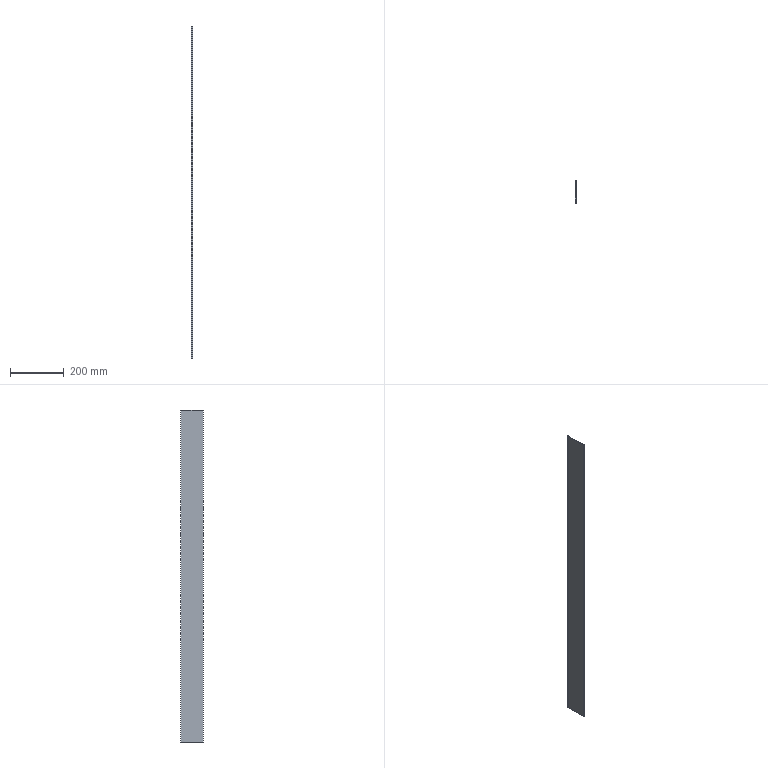Part | SolidWorks | features BaseBody 1 | 1 solid | 26 faces | box 4 x 85 x 1230 mm | volume 218982 mm3 | plane 18 | cylinder 8 | commonest cylinder face diameters 0.4 x4 1 x4
STEP:
#1=CARTESIAN_POINT('',(0.,0.,1230.));
#2=VERTEX_POINT('',#1);
#3=CARTESIAN_POINT('',(0.,0.,0.));
#4=VERTEX_POINT('',#3);
#5=CARTESIAN_POINT('',(0.,0.,1230.));
#6=DIRECTION('',(0.,0.,-1.));
#7=VECTOR('',#6,1000.);
#8=LINE('',#5,#7);
#9=EDGE_CURVE('',#2,#4,#8,.T.);
#10=ORIENTED_EDGE('',*,*,#9,.F.);
#11=CARTESIAN_POINT('',(0.,85.,1230.));
#12=VERTEX_POINT('',#11);
#13=CARTESIAN_POINT('',(0.,0.,1230.));
#14=DIRECTION('',(0.,-1.,0.));
#15=VECTOR('',#14,1000.);
#16=LINE('',#13,#15);
#17=EDGE_CURVE('',#12,#2,#16,.T.);
#18=ORIENTED_EDGE('',*,*,#17,.F.);
#19=CARTESIAN_POINT('',(0.,85.,0.));
#20=VERTEX_POINT('',#19);
#21=CARTESIAN_POINT('',(0.,85.,1230.));
#22=DIRECTION('',(0.,0.,1.));
#23=VECTOR('',#22,1000.);
#24=LINE('',#21,#23);
#25=EDGE_CURVE('',#20,#12,#24,.T.);
#26=ORIENTED_EDGE('',*,*,#25,.F.);
#27=CARTESIAN_POINT('',(0.,0.,0.));
#28=DIRECTION('',(0.,1.,0.));
#29=VECTOR('',#28,1000.);
#30=LINE('',#27,#29);
#31=EDGE_CURVE('',#4,#20,#30,.T.);
#32=ORIENTED_EDGE('',*,*,#31,.F.);
#33=EDGE_LOOP('',(#10,#18,#26,#32));
#34=FACE_OUTER_BOUND('',#33,.T.);
#35=CARTESIAN_POINT('',(0.,0.,1230.));
#36=DIRECTION('',(1.,0.,0.));
#37=DIRECTION('',(0.,0.,-1.));
#38=AXIS2_PLACEMENT_3D('',#35,#36,#37);
#39=PLANE('',#38);
#40=ADVANCED_FACE('',(#34),#39,.F.);
#41=CARTESIAN_POINT('',(1.2,3.,0.));
#42=VERTEX_POINT('',#41);
#43=CARTESIAN_POINT('',(1.,2.8,0.));
#44=VERTEX_POINT('',#43);
#45=CARTESIAN_POINT('',(1.2,2.8,0.));
#46=DIRECTION('',(0.,0.,1.));
#47=DIRECTION('',(-1.,0.,0.));
#48=AXIS2_PLACEMENT_3D('',#45,#46,#47);
#49=CIRCLE('',#48,0.2);
#50=EDGE_CURVE('',#42,#44,#49,.T.);
#51=ORIENTED_EDGE('',*,*,#50,.T.);
#52=CARTESIAN_POINT('',(1.,0.,0.));
#53=VERTEX_POINT('',#52);
#54=CARTESIAN_POINT('',(1.,82.2,0.));
#55=DIRECTION('',(0.,-1.,0.));
#56=VECTOR('',#55,1000.);
#57=LINE('',#54,#56);
#58=EDGE_CURVE('',#44,#53,#57,.T.);
#59=ORIENTED_EDGE('',*,*,#58,.T.);
#60=CARTESIAN_POINT('',(1.2,0.,0.));
#61=DIRECTION('',(-1.,0.,0.));
#62=VECTOR('',#61,1000.);
#63=LINE('',#60,#62);
#64=EDGE_CURVE('',#53,#4,#63,.T.);
#65=ORIENTED_EDGE('',*,*,#64,.T.);
#66=ORIENTED_EDGE('',*,*,#31,.T.);
#67=CARTESIAN_POINT('',(1.,85.,0.));
#68=VERTEX_POINT('',#67);
#69=CARTESIAN_POINT('',(1.2,85.,0.));
#70=DIRECTION('',(1.,0.,0.));
#71=VECTOR('',#70,1000.);
#72=LINE('',#69,#71);
#73=EDGE_CURVE('',#20,#68,#72,.T.);
#74=ORIENTED_EDGE('',*,*,#73,.T.);
#75=CARTESIAN_POINT('',(1.,82.2,0.));
#76=VERTEX_POINT('',#75);
#77=CARTESIAN_POINT('',(1.,82.2,0.));
#78=DIRECTION('',(0.,-1.,0.));
#79=VECTOR('',#78,1000.);
#80=LINE('',#77,#79);
#81=EDGE_CURVE('',#68,#76,#80,.T.);
#82=ORIENTED_EDGE('',*,*,#81,.T.);
#83=CARTESIAN_POINT('',(1.2,82.,0.));
#84=VERTEX_POINT('',#83);
#85=CARTESIAN_POINT('',(1.2,82.2,0.));
#86=DIRECTION('',(0.,0.,1.));
#87=DIRECTION('',(-1.,0.,0.));
#88=AXIS2_PLACEMENT_3D('',#85,#86,#87);
#89=CIRCLE('',#88,0.2);
#90=EDGE_CURVE('',#76,#84,#89,.T.);
#91=ORIENTED_EDGE('',*,*,#90,.T.);
#92=CARTESIAN_POINT('',(2.8,82.,0.));
#93=VERTEX_POINT('',#92);
#94=CARTESIAN_POINT('',(1.2,82.,0.));
#95=DIRECTION('',(1.,0.,0.));
#96=VECTOR('',#95,1000.);
#97=LINE('',#94,#96);
#98=EDGE_CURVE('',#84,#93,#97,.T.);
#99=ORIENTED_EDGE('',*,*,#98,.T.);
#100=CARTESIAN_POINT('',(3.,82.2,0.));
#101=VERTEX_POINT('',#100);
#102=CARTESIAN_POINT('',(2.8,82.2,0.));
#103=DIRECTION('',(0.,0.,1.));
#104=DIRECTION('',(-1.,0.,0.));
#105=AXIS2_PLACEMENT_3D('',#102,#103,#104);
#106=CIRCLE('',#105,0.2);
#107=EDGE_CURVE('',#93,#101,#106,.T.);
#108=ORIENTED_EDGE('',*,*,#107,.T.);
#109=CARTESIAN_POINT('',(3.,85.,0.));
#110=VERTEX_POINT('',#109);
#111=CARTESIAN_POINT('',(3.,82.2,0.));
#112=DIRECTION('',(0.,1.,0.));
#113=VECTOR('',#112,1000.);
#114=LINE('',#111,#113);
#115=EDGE_CURVE('',#101,#110,#114,.T.);
#116=ORIENTED_EDGE('',*,*,#115,.T.);
#117=CARTESIAN_POINT('',(4.,85.,0.));
#118=VERTEX_POINT('',#117);
#119=CARTESIAN_POINT('',(3.,85.,0.));
#120=DIRECTION('',(1.,0.,0.));
#121=VECTOR('',#120,1000.);
#122=LINE('',#119,#121);
#123=EDGE_CURVE('',#110,#118,#122,.T.);
#124=ORIENTED_EDGE('',*,*,#123,.T.);
#125=CARTESIAN_POINT('',(4.,80.5,0.));
#126=VERTEX_POINT('',#125);
#127=CARTESIAN_POINT('',(4.,82.2,0.));
#128=DIRECTION('',(0.,-1.,0.));
#129=VECTOR('',#128,1000.);
#130=LINE('',#127,#129);
#131=EDGE_CURVE('',#118,#126,#130,.T.);
#132=ORIENTED_EDGE('',*,*,#131,.T.);
#133=CARTESIAN_POINT('',(3.5,80.,0.));
#134=VERTEX_POINT('',#133);
#135=CARTESIAN_POINT('',(3.5,80.5,0.));
#136=DIRECTION('',(0.,0.,1.));
#137=DIRECTION('',(-1.,0.,0.));
#138=AXIS2_PLACEMENT_3D('',#135,#136,#137);
#139=CIRCLE('',#138,0.5);
#140=EDGE_CURVE('',#134,#126,#139,.T.);
#141=ORIENTED_EDGE('',*,*,#140,.F.);
#142=CARTESIAN_POINT('',(2.5,80.,0.));
#143=VERTEX_POINT('',#142);
#144=CARTESIAN_POINT('',(3.5,80.,0.));
#145=DIRECTION('',(-1.,0.,0.));
#146=VECTOR('',#145,1000.);
#147=LINE('',#144,#146);
#148=EDGE_CURVE('',#134,#143,#147,.T.);
#149=ORIENTED_EDGE('',*,*,#148,.T.);
#150=CARTESIAN_POINT('',(2.,79.5,0.));
#151=VERTEX_POINT('',#150);
#152=CARTESIAN_POINT('',(2.5,79.5,0.));
#153=DIRECTION('',(0.,0.,1.));
#154=DIRECTION('',(-1.,0.,0.));
#155=AXIS2_PLACEMENT_3D('',#152,#153,#154);
#156=CIRCLE('',#155,0.5);
#157=EDGE_CURVE('',#143,#151,#156,.T.);
#158=ORIENTED_EDGE('',*,*,#157,.T.);
#159=CARTESIAN_POINT('',(2.,5.5,0.));
#160=VERTEX_POINT('',#159);
#161=CARTESIAN_POINT('',(2.,82.2,0.));
#162=DIRECTION('',(0.,-1.,0.));
#163=VECTOR('',#162,1000.);
#164=LINE('',#161,#163);
#165=EDGE_CURVE('',#151,#160,#164,.T.);
#166=ORIENTED_EDGE('',*,*,#165,.T.);
#167=CARTESIAN_POINT('',(2.5,5.,0.));
#168=VERTEX_POINT('',#167);
#169=CARTESIAN_POINT('',(2.5,5.5,0.));
#170=DIRECTION('',(0.,0.,1.));
#171=DIRECTION('',(-1.,0.,0.));
#172=AXIS2_PLACEMENT_3D('',#169,#170,#171);
#173=CIRCLE('',#172,0.5);
#174=EDGE_CURVE('',#160,#168,#173,.T.);
#175=ORIENTED_EDGE('',*,*,#174,.T.);
#176=CARTESIAN_POINT('',(3.5,5.,0.));
#177=VERTEX_POINT('',#176);
#178=CARTESIAN_POINT('',(2.5,5.,0.));
#179=DIRECTION('',(1.,0.,0.));
#180=VECTOR('',#179,1000.);
#181=LINE('',#178,#180);
#182=EDGE_CURVE('',#168,#177,#181,.T.);
#183=ORIENTED_EDGE('',*,*,#182,.T.);
#184=CARTESIAN_POINT('',(4.,4.5,0.));
#185=VERTEX_POINT('',#184);
#186=CARTESIAN_POINT('',(3.5,4.5,0.));
#187=DIRECTION('',(0.,0.,1.));
#188=DIRECTION('',(-1.,0.,0.));
#189=AXIS2_PLACEMENT_3D('',#186,#187,#188);
#190=CIRCLE('',#189,0.5);
#191=EDGE_CURVE('',#185,#177,#190,.T.);
#192=ORIENTED_EDGE('',*,*,#191,.F.);
#193=CARTESIAN_POINT('',(4.,0.,0.));
#194=VERTEX_POINT('',#193);
#195=CARTESIAN_POINT('',(4.,82.2,0.));
#196=DIRECTION('',(0.,-1.,0.));
#197=VECTOR('',#196,1000.);
#198=LINE('',#195,#197);
#199=EDGE_CURVE('',#185,#194,#198,.T.);
#200=ORIENTED_EDGE('',*,*,#199,.T.);
#201=CARTESIAN_POINT('',(3.,0.,0.));
#202=VERTEX_POINT('',#201);
#203=CARTESIAN_POINT('',(4.,0.,0.));
#204=DIRECTION('',(-1.,0.,0.));
#205=VECTOR('',#204,1000.);
#206=LINE('',#203,#205);
#207=EDGE_CURVE('',#194,#202,#206,.T.);
#208=ORIENTED_EDGE('',*,*,#207,.T.);
#209=CARTESIAN_POINT('',(3.,2.8,0.));
#210=VERTEX_POINT('',#209);
#211=CARTESIAN_POINT('',(3.,82.2,0.));
#212=DIRECTION('',(0.,1.,0.));
#213=VECTOR('',#212,1000.);
#214=LINE('',#211,#213);
#215=EDGE_CURVE('',#202,#210,#214,.T.);
#216=ORIENTED_EDGE('',*,*,#215,.T.);
#217=CARTESIAN_POINT('',(2.8,3.,0.));
#218=VERTEX_POINT('',#217);
#219=CARTESIAN_POINT('',(2.8,2.8,0.));
#220=DIRECTION('',(0.,0.,1.));
#221=DIRECTION('',(-1.,0.,0.));
#222=AXIS2_PLACEMENT_3D('',#219,#220,#221);
#223=CIRCLE('',#222,0.2);
#224=EDGE_CURVE('',#210,#218,#223,.T.);
#225=ORIENTED_EDGE('',*,*,#224,.T.);
#226=CARTESIAN_POINT('',(2.8,3.,0.));
#227=DIRECTION('',(-1.,0.,0.));
#228=VECTOR('',#227,1000.);
#229=LINE('',#226,#228);
#230=EDGE_CURVE('',#218,#42,#229,.T.);
#231=ORIENTED_EDGE('',*,*,#230,.T.);
#232=EDGE_LOOP('',(#51,#59,#65,#66,#74,#82,#91,#99,#108,#116,#124,#132,#141,#149,#158,#166,#175,#183,#192,#200,#208,#216,#225,#231));
#233=FACE_OUTER_BOUND('',#232,.T.);
#234=CARTESIAN_POINT('',(1.2,82.2,0.));
#235=DIRECTION('',(0.,0.,-1.));
#236=DIRECTION('',(-1.,0.,0.));
#237=AXIS2_PLACEMENT_3D('',#234,#235,#236);
#238=PLANE('',#237);
#239=ADVANCED_FACE('',(#233),#238,.T.);
#240=CARTESIAN_POINT('',(1.,0.,1230.));
#241=VERTEX_POINT('',#240);
#242=CARTESIAN_POINT('',(1.,0.,1230.));
#243=DIRECTION('',(0.,0.,-1.));
#244=VECTOR('',#243,1000.);
#245=LINE('',#242,#244);
#246=EDGE_CURVE('',#241,#53,#245,.T.);
#247=ORIENTED_EDGE('',*,*,#246,.F.);
#248=CARTESIAN_POINT('',(1.,0.,1230.));
#249=DIRECTION('',(1.,0.,0.));
#250=VECTOR('',#249,1000.);
#251=LINE('',#248,#250);
#252=EDGE_CURVE('',#2,#241,#251,.T.);
#253=ORIENTED_EDGE('',*,*,#252,.F.);
#254=ORIENTED_EDGE('',*,*,#9,.T.);
#255=ORIENTED_EDGE('',*,*,#64,.F.);
#256=EDGE_LOOP('',(#247,#253,#254,#255));
#257=FACE_OUTER_BOUND('',#256,.T.);
#258=CARTESIAN_POINT('',(1.,0.,1230.));
#259=DIRECTION('',(0.,1.,0.));
#260=DIRECTION('',(-1.,0.,0.));
#261=AXIS2_PLACEMENT_3D('',#258,#259,#260);
#262=PLANE('',#261);
#263=ADVANCED_FACE('',(#257),#262,.F.);
#264=CARTESIAN_POINT('',(1.,2.8,1230.));
#265=VERTEX_POINT('',#264);
#266=CARTESIAN_POINT('',(1.,82.2,1230.));
#267=DIRECTION('',(0.,-1.,0.));
#268=VECTOR('',#267,1000.);
#269=LINE('',#266,#268);
#270=EDGE_CURVE('',#265,#241,#269,.T.);
#271=ORIENTED_EDGE('',*,*,#270,.F.);
#272=CARTESIAN_POINT('',(1.2,3.,1230.));
#273=VERTEX_POINT('',#272);
#274=CARTESIAN_POINT('',(1.2,2.8,1230.));
#275=DIRECTION('',(0.,0.,-1.));
#276=DIRECTION('',(-1.,0.,0.));
#277=AXIS2_PLACEMENT_3D('',#274,#275,#276);
#278=CIRCLE('',#277,0.2);
#279=EDGE_CURVE('',#265,#273,#278,.T.);
#280=ORIENTED_EDGE('',*,*,#279,.T.);
#281=CARTESIAN_POINT('',(2.8,3.,1230.));
#282=VERTEX_POINT('',#281);
#283=CARTESIAN_POINT('',(2.8,3.,1230.));
#284=DIRECTION('',(1.,0.,0.));
#285=VECTOR('',#284,1000.);
#286=LINE('',#283,#285);
#287=EDGE_CURVE('',#273,#282,#286,.T.);
#288=ORIENTED_EDGE('',*,*,#287,.T.);
#289=CARTESIAN_POINT('',(3.,2.8,1230.));
#290=VERTEX_POINT('',#289);
#291=CARTESIAN_POINT('',(2.8,2.8,1230.));
#292=DIRECTION('',(0.,0.,-1.));
#293=DIRECTION('',(-1.,0.,0.));
#294=AXIS2_PLACEMENT_3D('',#291,#292,#293);
#295=CIRCLE('',#294,0.2);
#296=EDGE_CURVE('',#282,#290,#295,.T.);
#297=ORIENTED_EDGE('',*,*,#296,.T.);
#298=CARTESIAN_POINT('',(3.,0.,1230.));
#299=VERTEX_POINT('',#298);
#300=CARTESIAN_POINT('',(3.,82.2,1230.));
#301=DIRECTION('',(0.,1.,0.));
#302=VECTOR('',#301,1000.);
#303=LINE('',#300,#302);
#304=EDGE_CURVE('',#299,#290,#303,.T.);
#305=ORIENTED_EDGE('',*,*,#304,.F.);
#306=CARTESIAN_POINT('',(4.,0.,1230.));
#307=VERTEX_POINT('',#306);
#308=CARTESIAN_POINT('',(4.,0.,1230.));
#309=DIRECTION('',(1.,0.,0.));
#310=VECTOR('',#309,1000.);
#311=LINE('',#308,#310);
#312=EDGE_CURVE('',#299,#307,#311,.T.);
#313=ORIENTED_EDGE('',*,*,#312,.T.);
#314=CARTESIAN_POINT('',(4.,4.5,1230.));
#315=VERTEX_POINT('',#314);
#316=CARTESIAN_POINT('',(4.,82.2,1230.));
#317=DIRECTION('',(0.,-1.,0.));
#318=VECTOR('',#317,1000.);
#319=LINE('',#316,#318);
#320=EDGE_CURVE('',#315,#307,#319,.T.);
#321=ORIENTED_EDGE('',*,*,#320,.F.);
#322=CARTESIAN_POINT('',(3.5,5.,1230.));
#323=VERTEX_POINT('',#322);
#324=CARTESIAN_POINT('',(3.5,4.5,1230.));
#325=DIRECTION('',(0.,0.,-1.));
#326=DIRECTION('',(-1.,0.,0.));
#327=AXIS2_PLACEMENT_3D('',#324,#325,#326);
#328=CIRCLE('',#327,0.5);
#329=EDGE_CURVE('',#323,#315,#328,.T.);
#330=ORIENTED_EDGE('',*,*,#329,.F.);
#331=CARTESIAN_POINT('',(2.5,5.,1230.));
#332=VERTEX_POINT('',#331);
#333=CARTESIAN_POINT('',(2.5,5.,1230.));
#334=DIRECTION('',(-1.,0.,0.));
#335=VECTOR('',#334,1000.);
#336=LINE('',#333,#335);
#337=EDGE_CURVE('',#323,#332,#336,.T.);
#338=ORIENTED_EDGE('',*,*,#337,.T.);
#339=CARTESIAN_POINT('',(2.,5.5,1230.));
#340=VERTEX_POINT('',#339);
#341=CARTESIAN_POINT('',(2.5,5.5,1230.));
#342=DIRECTION('',(0.,0.,-1.));
#343=DIRECTION('',(-1.,0.,0.));
#344=AXIS2_PLACEMENT_3D('',#341,#342,#343);
#345=CIRCLE('',#344,0.5);
#346=EDGE_CURVE('',#332,#340,#345,.T.);
#347=ORIENTED_EDGE('',*,*,#346,.T.);
#348=CARTESIAN_POINT('',(2.,79.5,1230.));
#349=VERTEX_POINT('',#348);
#350=CARTESIAN_POINT('',(2.,82.2,1230.));
#351=DIRECTION('',(0.,-1.,0.));
#352=VECTOR('',#351,1000.);
#353=LINE('',#350,#352);
#354=EDGE_CURVE('',#349,#340,#353,.T.);
#355=ORIENTED_EDGE('',*,*,#354,.F.);
#356=CARTESIAN_POINT('',(2.5,80.,1230.));
#357=VERTEX_POINT('',#356);
#358=CARTESIAN_POINT('',(2.5,79.5,1230.));
#359=DIRECTION('',(0.,0.,-1.));
#360=DIRECTION('',(-1.,0.,0.));
#361=AXIS2_PLACEMENT_3D('',#358,#359,#360);
#362=CIRCLE('',#361,0.5);
#363=EDGE_CURVE('',#349,#357,#362,.T.);
#364=ORIENTED_EDGE('',*,*,#363,.T.);
#365=CARTESIAN_POINT('',(3.5,80.,1230.));
#366=VERTEX_POINT('',#365);
#367=CARTESIAN_POINT('',(3.5,80.,1230.));
#368=DIRECTION('',(1.,0.,0.));
#369=VECTOR('',#368,1000.);
#370=LINE('',#367,#369);
#371=EDGE_CURVE('',#357,#366,#370,.T.);
#372=ORIENTED_EDGE('',*,*,#371,.T.);
#373=CARTESIAN_POINT('',(4.,80.5,1230.));
#374=VERTEX_POINT('',#373);
#375=CARTESIAN_POINT('',(3.5,80.5,1230.));
#376=DIRECTION('',(0.,0.,-1.));
#377=DIRECTION('',(-1.,0.,0.));
#378=AXIS2_PLACEMENT_3D('',#375,#376,#377);
#379=CIRCLE('',#378,0.5);
#380=EDGE_CURVE('',#374,#366,#379,.T.);
#381=ORIENTED_EDGE('',*,*,#380,.F.);
#382=CARTESIAN_POINT('',(4.,85.,1230.));
#383=VERTEX_POINT('',#382);
#384=CARTESIAN_POINT('',(4.,82.2,1230.));
#385=DIRECTION('',(0.,-1.,0.));
#386=VECTOR('',#385,1000.);
#387=LINE('',#384,#386);
#388=EDGE_CURVE('',#383,#374,#387,.T.);
#389=ORIENTED_EDGE('',*,*,#388,.F.);
#390=CARTESIAN_POINT('',(3.,85.,1230.));
#391=VERTEX_POINT('',#390);
#392=CARTESIAN_POINT('',(3.,85.,1230.));
#393=DIRECTION('',(-1.,0.,0.));
#394=VECTOR('',#393,1000.);
#395=LINE('',#392,#394);
#396=EDGE_CURVE('',#383,#391,#395,.T.);
#397=ORIENTED_EDGE('',*,*,#396,.T.);
#398=CARTESIAN_POINT('',(3.,82.2,1230.));
#399=VERTEX_POINT('',#398);
#400=CARTESIAN_POINT('',(3.,82.2,1230.));
#401=DIRECTION('',(0.,1.,0.));
#402=VECTOR('',#401,1000.);
#403=LINE('',#400,#402);
#404=EDGE_CURVE('',#399,#391,#403,.T.);
#405=ORIENTED_EDGE('',*,*,#404,.F.);
#406=CARTESIAN_POINT('',(2.8,82.,1230.));
#407=VERTEX_POINT('',#406);
#408=CARTESIAN_POINT('',(2.8,82.2,1230.));
#409=DIRECTION('',(0.,0.,-1.));
#410=DIRECTION('',(-1.,0.,0.));
#411=AXIS2_PLACEMENT_3D('',#408,#409,#410);
#412=CIRCLE('',#411,0.2);
#413=EDGE_CURVE('',#399,#407,#412,.T.);
#414=ORIENTED_EDGE('',*,*,#413,.T.);
#415=CARTESIAN_POINT('',(1.2,82.,1230.));
#416=VERTEX_POINT('',#415);
#417=CARTESIAN_POINT('',(1.2,82.,1230.));
#418=DIRECTION('',(-1.,0.,0.));
#419=VECTOR('',#418,1000.);
#420=LINE('',#417,#419);
#421=EDGE_CURVE('',#407,#416,#420,.T.);
#422=ORIENTED_EDGE('',*,*,#421,.T.);
#423=CARTESIAN_POINT('',(1.,82.2,1230.));
#424=VERTEX_POINT('',#423);
#425=CARTESIAN_POINT('',(1.2,82.2,1230.));
#426=DIRECTION('',(0.,0.,-1.));
#427=DIRECTION('',(-1.,0.,0.));
#428=AXIS2_PLACEMENT_3D('',#425,#426,#427);
#429=CIRCLE('',#428,0.2);
#430=EDGE_CURVE('',#416,#424,#429,.T.);
#431=ORIENTED_EDGE('',*,*,#430,.T.);
#432=CARTESIAN_POINT('',(1.,85.,1230.));
#433=VERTEX_POINT('',#432);
#434=CARTESIAN_POINT('',(1.,82.2,1230.));
#435=DIRECTION('',(0.,-1.,0.));
#436=VECTOR('',#435,1000.);
#437=LINE('',#434,#436);
#438=EDGE_CURVE('',#433,#424,#437,.T.);
#439=ORIENTED_EDGE('',*,*,#438,.F.);
#440=CARTESIAN_POINT('',(1.2,85.,1230.));
#441=DIRECTION('',(1.,0.,0.));
#442=VECTOR('',#441,1000.);
#443=LINE('',#440,#442);
#444=EDGE_CURVE('',#12,#433,#443,.T.);
#445=ORIENTED_EDGE('',*,*,#444,.F.);
#446=ORIENTED_EDGE('',*,*,#17,.T.);
#447=ORIENTED_EDGE('',*,*,#252,.T.);
#448=EDGE_LOOP('',(#271,#280,#288,#297,#305,#313,#321,#330,#338,#347,#355,#364,#372,#381,#389,#397,#405,#414,#422,#431,#439,#445,#446,#447));
#449=FACE_OUTER_BOUND('',#448,.T.);
#450=CARTESIAN_POINT('',(1.2,82.2,1230.));
#451=DIRECTION('',(0.,0.,-1.));
#452=DIRECTION('',(-1.,0.,0.));
#453=AXIS2_PLACEMENT_3D('',#450,#451,#452);
#454=PLANE('',#453);
#455=ADVANCED_FACE('',(#449),#454,.F.);
#456=ORIENTED_EDGE('',*,*,#25,.T.);
#457=ORIENTED_EDGE('',*,*,#444,.T.);
#458=CARTESIAN_POINT('',(1.,85.,1230.));
#459=DIRECTION('',(0.,0.,1.));
#460=VECTOR('',#459,1000.);
#461=LINE('',#458,#460);
#462=EDGE_CURVE('',#68,#433,#461,.T.);
#463=ORIENTED_EDGE('',*,*,#462,.F.);
#464=ORIENTED_EDGE('',*,*,#73,.F.);
#465=EDGE_LOOP('',(#456,#457,#463,#464));
#466=FACE_OUTER_BOUND('',#465,.T.);
#467=CARTESIAN_POINT('',(0.,85.,1230.));
#468=DIRECTION('',(0.,-1.,0.));
#469=DIRECTION('',(0.,0.,-1.));
#470=AXIS2_PLACEMENT_3D('',#467,#468,#469);
#471=PLANE('',#470);
#472=ADVANCED_FACE('',(#466),#471,.F.);
#473=CARTESIAN_POINT('',(1.,2.8,1230.));
#474=DIRECTION('',(0.,0.,-1.));
#475=VECTOR('',#474,1000.);
#476=LINE('',#473,#475);
#477=EDGE_CURVE('',#265,#44,#476,.T.);
#478=ORIENTED_EDGE('',*,*,#477,.F.);
#479=ORIENTED_EDGE('',*,*,#270,.T.);
#480=ORIENTED_EDGE('',*,*,#246,.T.);
#481=ORIENTED_EDGE('',*,*,#58,.F.);
#482=EDGE_LOOP('',(#478,#479,#480,#481));
#483=FACE_OUTER_BOUND('',#482,.T.);
#484=CARTESIAN_POINT('',(1.,2.8,1230.));
#485=DIRECTION('',(-1.,0.,0.));
#486=DIRECTION('',(0.,-1.,0.));
#487=AXIS2_PLACEMENT_3D('',#484,#485,#486);
#488=PLANE('',#487);
#489=ADVANCED_FACE('',(#483),#488,.F.);
#490=CARTESIAN_POINT('',(3.,0.,1230.));
#491=DIRECTION('',(0.,0.,-1.));
#492=VECTOR('',#491,1000.);
#493=LINE('',#490,#492);
#494=EDGE_CURVE('',#299,#202,#493,.T.);
#495=ORIENTED_EDGE('',*,*,#494,.F.);
#496=ORIENTED_EDGE('',*,*,#304,.T.);
#497=CARTESIAN_POINT('',(3.,2.8,1230.));
#498=DIRECTION('',(0.,0.,1.));
#499=VECTOR('',#498,1000.);
#500=LINE('',#497,#499);
#501=EDGE_CURVE('',#210,#290,#500,.T.);
#502=ORIENTED_EDGE('',*,*,#501,.F.);
#503=ORIENTED_EDGE('',*,*,#215,.F.);
#504=EDGE_LOOP('',(#495,#496,#502,#503));
#505=FACE_OUTER_BOUND('',#504,.T.);
#506=CARTESIAN_POINT('',(3.,0.,1230.));
#507=DIRECTION('',(1.,0.,0.));
#508=DIRECTION('',(0.,0.,-1.));
#509=AXIS2_PLACEMENT_3D('',#506,#507,#508);
#510=PLANE('',#509);
#511=ADVANCED_FACE('',(#505),#510,.F.);
#512=CARTESIAN_POINT('',(4.,4.5,1230.));
#513=DIRECTION('',(0.,0.,-1.));
#514=VECTOR('',#513,1000.);
#515=LINE('',#512,#514);
#516=EDGE_CURVE('',#315,#185,#515,.T.);
#517=ORIENTED_EDGE('',*,*,#516,.F.);
#518=ORIENTED_EDGE('',*,*,#320,.T.);
#519=CARTESIAN_POINT('',(4.,0.,1230.));
#520=DIRECTION('',(0.,0.,1.));
#521=VECTOR('',#520,1000.);
#522=LINE('',#519,#521);
#523=EDGE_CURVE('',#194,#307,#522,.T.);
#524=ORIENTED_EDGE('',*,*,#523,.F.);
#525=ORIENTED_EDGE('',*,*,#199,.F.);
#526=EDGE_LOOP('',(#517,#518,#524,#525));
#527=FACE_OUTER_BOUND('',#526,.T.);
#528=CARTESIAN_POINT('',(4.,4.5,1230.));
#529=DIRECTION('',(-1.,0.,0.));
#530=DIRECTION('',(0.,-1.,0.));
#531=AXIS2_PLACEMENT_3D('',#528,#529,#530);
#532=PLANE('',#531);
#533=ADVANCED_FACE('',(#527),#532,.F.);
#534=CARTESIAN_POINT('',(2.,79.5,1230.));
#535=DIRECTION('',(0.,0.,-1.));
#536=VECTOR('',#535,1000.);
#537=LINE('',#534,#536);
#538=EDGE_CURVE('',#349,#151,#537,.T.);
#539=ORIENTED_EDGE('',*,*,#538,.F.);
#540=ORIENTED_EDGE('',*,*,#354,.T.);
#541=CARTESIAN_POINT('',(2.,5.5,1230.));
#542=DIRECTION('',(0.,0.,1.));
#543=VECTOR('',#542,1000.);
#544=LINE('',#541,#543);
#545=EDGE_CURVE('',#160,#340,#544,.T.);
#546=ORIENTED_EDGE('',*,*,#545,.F.);
#547=ORIENTED_EDGE('',*,*,#165,.F.);
#548=EDGE_LOOP('',(#539,#540,#546,#547));
#549=FACE_OUTER_BOUND('',#548,.T.);
#550=CARTESIAN_POINT('',(2.,79.5,1230.));
#551=DIRECTION('',(-1.,0.,0.));
#552=DIRECTION('',(0.,-1.,0.));
#553=AXIS2_PLACEMENT_3D('',#550,#551,#552);
#554=PLANE('',#553);
#555=ADVANCED_FACE('',(#549),#554,.F.);
#556=CARTESIAN_POINT('',(4.,85.,1230.));
#557=DIRECTION('',(0.,0.,-1.));
#558=VECTOR('',#557,1000.);
#559=LINE('',#556,#558);
#560=EDGE_CURVE('',#383,#118,#559,.T.);
#561=ORIENTED_EDGE('',*,*,#560,.F.);
#562=ORIENTED_EDGE('',*,*,#388,.T.);
#563=CARTESIAN_POINT('',(4.,80.5,1230.));
#564=DIRECTION('',(0.,0.,1.));
#565=VECTOR('',#564,1000.);
#566=LINE('',#563,#565);
#567=EDGE_CURVE('',#126,#374,#566,.T.);
#568=ORIENTED_EDGE('',*,*,#567,.F.);
#569=ORIENTED_EDGE('',*,*,#131,.F.);
#570=EDGE_LOOP('',(#561,#562,#568,#569));
#571=FACE_OUTER_BOUND('',#570,.T.);
#572=CARTESIAN_POINT('',(4.,85.,1230.));
#573=DIRECTION('',(-1.,0.,0.));
#574=DIRECTION('',(0.,0.,1.));
#575=AXIS2_PLACEMENT_3D('',#572,#573,#574);
#576=PLANE('',#575);
#577=ADVANCED_FACE('',(#571),#576,.F.);
#578=CARTESIAN_POINT('',(3.,82.2,1230.));
#579=DIRECTION('',(0.,0.,-1.));
#580=VECTOR('',#579,1000.);
#581=LINE('',#578,#580);
#582=EDGE_CURVE('',#399,#101,#581,.T.);
#583=ORIENTED_EDGE('',*,*,#582,.F.);
#584=ORIENTED_EDGE('',*,*,#404,.T.);
#585=CARTESIAN_POINT('',(3.,85.,1230.));
#586=DIRECTION('',(0.,0.,1.));
#587=VECTOR('',#586,1000.);
#588=LINE('',#585,#587);
#589=EDGE_CURVE('',#110,#391,#588,.T.);
#590=ORIENTED_EDGE('',*,*,#589,.F.);
#591=ORIENTED_EDGE('',*,*,#115,.F.);
#592=EDGE_LOOP('',(#583,#584,#590,#591));
#593=FACE_OUTER_BOUND('',#592,.T.);
#594=CARTESIAN_POINT('',(3.,82.2,1230.));
#595=DIRECTION('',(1.,0.,0.));
#596=DIRECTION('',(0.,0.,-1.));
#597=AXIS2_PLACEMENT_3D('',#594,#595,#596);
#598=PLANE('',#597);
#599=ADVANCED_FACE('',(#593),#598,.F.);
#600=ORIENTED_EDGE('',*,*,#462,.T.);
#601=ORIENTED_EDGE('',*,*,#438,.T.);
#602=CARTESIAN_POINT('',(1.,82.2,1230.));
#603=DIRECTION('',(0.,0.,1.));
#604=VECTOR('',#603,1000.);
#605=LINE('',#602,#604);
#606=EDGE_CURVE('',#76,#424,#605,.T.);
#607=ORIENTED_EDGE('',*,*,#606,.F.);
#608=ORIENTED_EDGE('',*,*,#81,.F.);
#609=EDGE_LOOP('',(#600,#601,#607,#608));
#610=FACE_OUTER_BOUND('',#609,.T.);
#611=CARTESIAN_POINT('',(1.,85.,1230.));
#612=DIRECTION('',(-1.,0.,0.));
#613=DIRECTION('',(0.,-1.,0.));
#614=AXIS2_PLACEMENT_3D('',#611,#612,#613);
#615=PLANE('',#614);
#616=ADVANCED_FACE('',(#610),#615,.F.);
#617=CARTESIAN_POINT('',(1.2,3.,1230.));
#618=DIRECTION('',(0.,0.,-1.));
#619=VECTOR('',#618,1000.);
#620=LINE('',#617,#619);
#621=EDGE_CURVE('',#273,#42,#620,.T.);
#622=ORIENTED_EDGE('',*,*,#621,.F.);
#623=ORIENTED_EDGE('',*,*,#279,.F.);
#624=ORIENTED_EDGE('',*,*,#477,.T.);
#625=ORIENTED_EDGE('',*,*,#50,.F.);
#626=EDGE_LOOP('',(#622,#623,#624,#625));
#627=FACE_OUTER_BOUND('',#626,.T.);
#628=CARTESIAN_POINT('',(1.2,2.8,1230.));
#629=DIRECTION('',(0.,0.,-1.));
#630=DIRECTION('',(-1.,0.,0.));
#631=AXIS2_PLACEMENT_3D('',#628,#629,#630);
#632=CYLINDRICAL_SURFACE('',#631,0.2);
#633=ADVANCED_FACE('',(#627),#632,.F.);
#634=ORIENTED_EDGE('',*,*,#523,.T.);
#635=ORIENTED_EDGE('',*,*,#312,.F.);
#636=ORIENTED_EDGE('',*,*,#494,.T.);
#637=ORIENTED_EDGE('',*,*,#207,.F.);
#638=EDGE_LOOP('',(#634,#635,#636,#637));
#639=FACE_OUTER_BOUND('',#638,.T.);
#640=CARTESIAN_POINT('',(4.,0.,1230.));
#641=DIRECTION('',(0.,1.,0.));
#642=DIRECTION('',(-1.,0.,0.));
#643=AXIS2_PLACEMENT_3D('',#640,#641,#642);
#644=PLANE('',#643);
#645=ADVANCED_FACE('',(#639),#644,.F.);
#646=ORIENTED_EDGE('',*,*,#501,.T.);
#647=ORIENTED_EDGE('',*,*,#296,.F.);
#648=CARTESIAN_POINT('',(2.8,3.,1230.));
#649=DIRECTION('',(0.,0.,1.));
#650=VECTOR('',#649,1000.);
#651=LINE('',#648,#650);
#652=EDGE_CURVE('',#218,#282,#651,.T.);
#653=ORIENTED_EDGE('',*,*,#652,.F.);
#654=ORIENTED_EDGE('',*,*,#224,.F.);
#655=EDGE_LOOP('',(#646,#647,#653,#654));
#656=FACE_OUTER_BOUND('',#655,.T.);
#657=CARTESIAN_POINT('',(2.8,2.8,1230.));
#658=DIRECTION('',(0.,0.,-1.));
#659=DIRECTION('',(-1.,0.,0.));
#660=AXIS2_PLACEMENT_3D('',#657,#658,#659);
#661=CYLINDRICAL_SURFACE('',#660,0.2);
#662=ADVANCED_FACE('',(#656),#661,.F.);
#663=ORIENTED_EDGE('',*,*,#329,.T.);
#664=ORIENTED_EDGE('',*,*,#516,.T.);
#665=ORIENTED_EDGE('',*,*,#191,.T.);
#666=CARTESIAN_POINT('',(3.5,5.,1230.));
#667=DIRECTION('',(0.,0.,1.));
#668=VECTOR('',#667,1000.);
#669=LINE('',#666,#668);
#670=EDGE_CURVE('',#177,#323,#669,.T.);
#671=ORIENTED_EDGE('',*,*,#670,.T.);
#672=EDGE_LOOP('',(#663,#664,#665,#671));
#673=FACE_OUTER_BOUND('',#672,.T.);
#674=CARTESIAN_POINT('',(3.5,4.5,1230.));
#675=DIRECTION('',(0.,0.,-1.));
#676=DIRECTION('',(-1.,0.,0.));
#677=AXIS2_PLACEMENT_3D('',#674,#675,#676);
#678=CYLINDRICAL_SURFACE('',#677,0.5);
#679=ADVANCED_FACE('',(#673),#678,.T.);
#680=CARTESIAN_POINT('',(2.5,80.,1230.));
#681=DIRECTION('',(0.,0.,-1.));
#682=VECTOR('',#681,1000.);
#683=LINE('',#680,#682);
#684=EDGE_CURVE('',#357,#143,#683,.T.);
#685=ORIENTED_EDGE('',*,*,#684,.F.);
#686=ORIENTED_EDGE('',*,*,#363,.F.);
#687=ORIENTED_EDGE('',*,*,#538,.T.);
#688=ORIENTED_EDGE('',*,*,#157,.F.);
#689=EDGE_LOOP('',(#685,#686,#687,#688));
#690=FACE_OUTER_BOUND('',#689,.T.);
#691=CARTESIAN_POINT('',(2.5,79.5,1230.));
#692=DIRECTION('',(0.,0.,-1.));
#693=DIRECTION('',(-1.,0.,0.));
#694=AXIS2_PLACEMENT_3D('',#691,#692,#693);
#695=CYLINDRICAL_SURFACE('',#694,0.5);
#696=ADVANCED_FACE('',(#690),#695,.F.);
#697=ORIENTED_EDGE('',*,*,#545,.T.);
#698=ORIENTED_EDGE('',*,*,#346,.F.);
#699=CARTESIAN_POINT('',(2.5,5.,1230.));
#700=DIRECTION('',(0.,0.,1.));
#701=VECTOR('',#700,1000.);
#702=LINE('',#699,#701);
#703=EDGE_CURVE('',#168,#332,#702,.T.);
#704=ORIENTED_EDGE('',*,*,#703,.F.);
#705=ORIENTED_EDGE('',*,*,#174,.F.);
#706=EDGE_LOOP('',(#697,#698,#704,#705));
#707=FACE_OUTER_BOUND('',#706,.T.);
#708=CARTESIAN_POINT('',(2.5,5.5,1230.));
#709=DIRECTION('',(0.,0.,-1.));
#710=DIRECTION('',(-1.,0.,0.));
#711=AXIS2_PLACEMENT_3D('',#708,#709,#710);
#712=CYLINDRICAL_SURFACE('',#711,0.5);
#713=ADVANCED_FACE('',(#707),#712,.F.);
#714=ORIENTED_EDGE('',*,*,#589,.T.);
#715=ORIENTED_EDGE('',*,*,#396,.F.);
#716=ORIENTED_EDGE('',*,*,#560,.T.);
#717=ORIENTED_EDGE('',*,*,#123,.F.);
#718=EDGE_LOOP('',(#714,#715,#716,#717));
#719=FACE_OUTER_BOUND('',#718,.T.);
#720=CARTESIAN_POINT('',(3.,85.,1230.));
#721=DIRECTION('',(0.,-1.,0.));
#722=DIRECTION('',(0.,0.,-1.));
#723=AXIS2_PLACEMENT_3D('',#720,#721,#722);
#724=PLANE('',#723);
#725=ADVANCED_FACE('',(#719),#724,.F.);
#726=ORIENTED_EDGE('',*,*,#380,.T.);
#727=CARTESIAN_POINT('',(3.5,80.,1230.));
#728=DIRECTION('',(0.,0.,-1.));
#729=VECTOR('',#728,1000.);
#730=LINE('',#727,#729);
#731=EDGE_CURVE('',#366,#134,#730,.T.);
#732=ORIENTED_EDGE('',*,*,#731,.T.);
#733=ORIENTED_EDGE('',*,*,#140,.T.);
#734=ORIENTED_EDGE('',*,*,#567,.T.);
#735=EDGE_LOOP('',(#726,#732,#733,#734));
#736=FACE_OUTER_BOUND('',#735,.T.);
#737=CARTESIAN_POINT('',(3.5,80.5,1230.));
#738=DIRECTION('',(0.,0.,-1.));
#739=DIRECTION('',(-1.,0.,0.));
#740=AXIS2_PLACEMENT_3D('',#737,#738,#739);
#741=CYLINDRICAL_SURFACE('',#740,0.5);
#742=ADVANCED_FACE('',(#736),#741,.T.);
#743=CARTESIAN_POINT('',(2.8,82.,1230.));
#744=DIRECTION('',(0.,0.,-1.));
#745=VECTOR('',#744,1000.);
#746=LINE('',#743,#745);
#747=EDGE_CURVE('',#407,#93,#746,.T.);
#748=ORIENTED_EDGE('',*,*,#747,.F.);
#749=ORIENTED_EDGE('',*,*,#413,.F.);
#750=ORIENTED_EDGE('',*,*,#582,.T.);
#751=ORIENTED_EDGE('',*,*,#107,.F.);
#752=EDGE_LOOP('',(#748,#749,#750,#751));
#753=FACE_OUTER_BOUND('',#752,.T.);
#754=CARTESIAN_POINT('',(2.8,82.2,1230.));
#755=DIRECTION('',(0.,0.,-1.));
#756=DIRECTION('',(-1.,0.,0.));
#757=AXIS2_PLACEMENT_3D('',#754,#755,#756);
#758=CYLINDRICAL_SURFACE('',#757,0.2);
#759=ADVANCED_FACE('',(#753),#758,.F.);
#760=ORIENTED_EDGE('',*,*,#606,.T.);
#761=ORIENTED_EDGE('',*,*,#430,.F.);
#762=CARTESIAN_POINT('',(1.2,82.,1230.));
#763=DIRECTION('',(0.,0.,1.));
#764=VECTOR('',#763,1000.);
#765=LINE('',#762,#764);
#766=EDGE_CURVE('',#84,#416,#765,.T.);
#767=ORIENTED_EDGE('',*,*,#766,.F.);
#768=ORIENTED_EDGE('',*,*,#90,.F.);
#769=EDGE_LOOP('',(#760,#761,#767,#768));
#770=FACE_OUTER_BOUND('',#769,.T.);
#771=CARTESIAN_POINT('',(1.2,82.2,1230.));
#772=DIRECTION('',(0.,0.,-1.));
#773=DIRECTION('',(-1.,0.,0.));
#774=AXIS2_PLACEMENT_3D('',#771,#772,#773);
#775=CYLINDRICAL_SURFACE('',#774,0.2);
#776=ADVANCED_FACE('',(#770),#775,.F.);
#777=ORIENTED_EDGE('',*,*,#652,.T.);
#778=ORIENTED_EDGE('',*,*,#287,.F.);
#779=ORIENTED_EDGE('',*,*,#621,.T.);
#780=ORIENTED_EDGE('',*,*,#230,.F.);
#781=EDGE_LOOP('',(#777,#778,#779,#780));
#782=FACE_OUTER_BOUND('',#781,.T.);
#783=CARTESIAN_POINT('',(2.8,3.,1230.));
#784=DIRECTION('',(0.,1.,0.));
#785=DIRECTION('',(0.,0.,1.));
#786=AXIS2_PLACEMENT_3D('',#783,#784,#785);
#787=PLANE('',#786);
#788=ADVANCED_FACE('',(#782),#787,.F.);
#789=ORIENTED_EDGE('',*,*,#703,.T.);
#790=ORIENTED_EDGE('',*,*,#337,.F.);
#791=ORIENTED_EDGE('',*,*,#670,.F.);
#792=ORIENTED_EDGE('',*,*,#182,.F.);
#793=EDGE_LOOP('',(#789,#790,#791,#792));
#794=FACE_OUTER_BOUND('',#793,.T.);
#795=CARTESIAN_POINT('',(2.5,5.,1230.));
#796=DIRECTION('',(0.,-1.,0.));
#797=DIRECTION('',(1.,0.,0.));
#798=AXIS2_PLACEMENT_3D('',#795,#796,#797);
#799=PLANE('',#798);
#800=ADVANCED_FACE('',(#794),#799,.F.);
#801=ORIENTED_EDGE('',*,*,#731,.F.);
#802=ORIENTED_EDGE('',*,*,#371,.F.);
#803=ORIENTED_EDGE('',*,*,#684,.T.);
#804=ORIENTED_EDGE('',*,*,#148,.F.);
#805=EDGE_LOOP('',(#801,#802,#803,#804));
#806=FACE_OUTER_BOUND('',#805,.T.);
#807=CARTESIAN_POINT('',(3.5,80.,1230.));
#808=DIRECTION('',(0.,1.,0.));
#809=DIRECTION('',(0.,0.,1.));
#810=AXIS2_PLACEMENT_3D('',#807,#808,#809);
#811=PLANE('',#810);
#812=ADVANCED_FACE('',(#806),#811,.F.);
#813=ORIENTED_EDGE('',*,*,#766,.T.);
#814=ORIENTED_EDGE('',*,*,#421,.F.);
#815=ORIENTED_EDGE('',*,*,#747,.T.);
#816=ORIENTED_EDGE('',*,*,#98,.F.);
#817=EDGE_LOOP('',(#813,#814,#815,#816));
#818=FACE_OUTER_BOUND('',#817,.T.);
#819=CARTESIAN_POINT('',(1.2,82.,1230.));
#820=DIRECTION('',(0.,-1.,0.));
#821=DIRECTION('',(0.,0.,-1.));
#822=AXIS2_PLACEMENT_3D('',#819,#820,#821);
#823=PLANE('',#822);
#824=ADVANCED_FACE('',(#818),#823,.F.);
#825=CLOSED_SHELL('',(#40,#239,#263,#455,#472,#489,#511,#533,#555,#577,#599,#616,#633,#645,#662,#679,#696,#713,#725,#742,#759,#776,#788,#800,#812,#824));
#826=MANIFOLD_SOLID_BREP('',#825);
#827=CARTESIAN_POINT('',(0.,0.,0.));
#828=DIRECTION('',(0.,0.,1.));
#829=DIRECTION('',(1.,0.,0.));
#830=AXIS2_PLACEMENT_3D('',#827,#828,#829);
#831=(LENGTH_UNIT()NAMED_UNIT(*)SI_UNIT(.MILLI.,.METRE.));
#832=UNCERTAINTY_MEASURE_WITH_UNIT(LENGTH_MEASURE(0.00001),#831,'','');
#833=(NAMED_UNIT(*)PLANE_ANGLE_UNIT()SI_UNIT($,.RADIAN.));
#834=(NAMED_UNIT(*)SI_UNIT($,.STERADIAN.)SOLID_ANGLE_UNIT());
#835=(GEOMETRIC_REPRESENTATION_CONTEXT(3)GLOBAL_UNCERTAINTY_ASSIGNED_CONTEXT((#832))GLOBAL_UNIT_ASSIGNED_CONTEXT((#831,#833,#834))REPRESENTATION_CONTEXT('',''));
#836=ADVANCED_BREP_SHAPE_REPRESENTATION('',(#826,#830),#835);